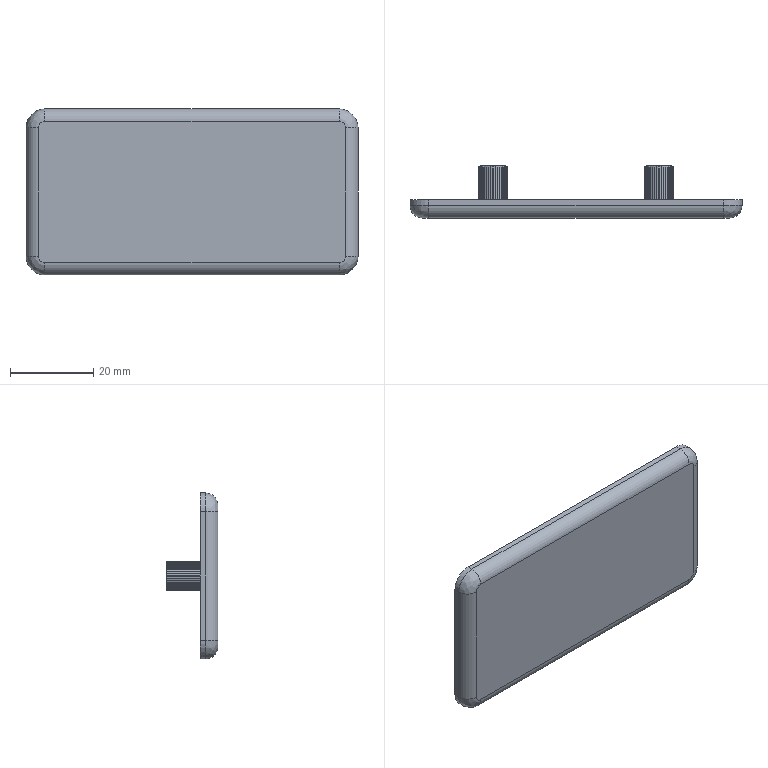Part | STEP file | End Cover Panel MK-EC-B-4080x4.3 | 1 solid | 259 faces | box 80 x 12.5 x 40 mm | volume 10356 mm3 | cylinder 128 | plane 119 | torus 8 | other 4 | commonest cylinder face diameters 6.6 x48 7 x46 2 x8 4.1 x8 9 x8 4.9 x6